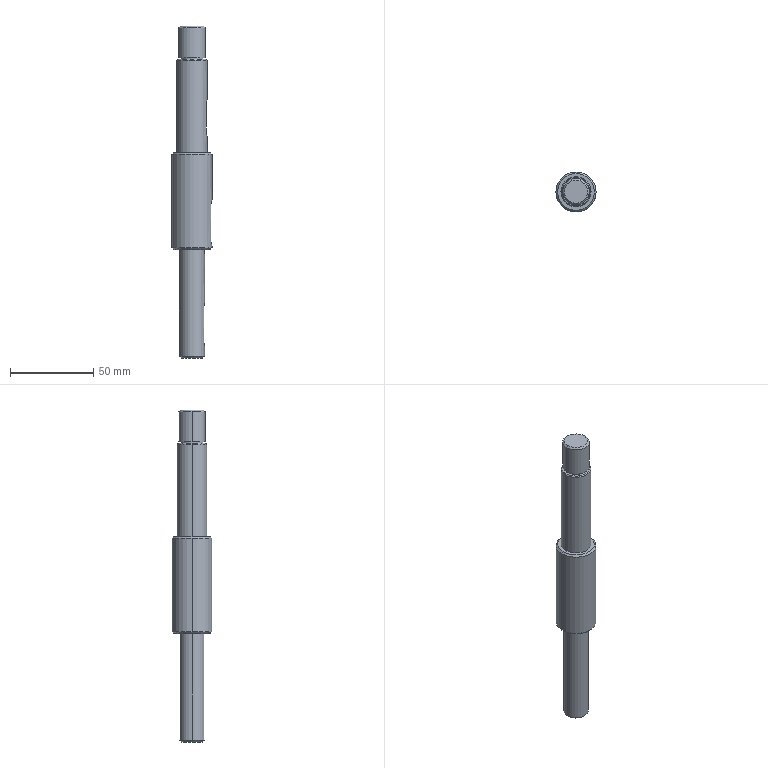Part | SolidWorks | features ICE 8, Chamfer 5, MoveFace 2, Cut 1, Revolution 1 | 1 solid | 44 faces | box 24 x 24 x 199 mm | volume 54258 mm3 | cylinder 19 | plane 15 | cone 10 | commonest cylinder face diameters 5 x3 6 x3 8 x3 13.5 x2 15 x2 16 x2
STEP:
#1=CARTESIAN_POINT('',(4.5,0.,-191.5));
#2=VERTEX_POINT('',#1);
#3=CARTESIAN_POINT('',(4.5,2.5,-189.));
#4=VERTEX_POINT('',#3);
#5=CARTESIAN_POINT('',(4.5,0.,-189.));
#6=DIRECTION('',(1.,0.,0.));
#7=DIRECTION('',(0.,0.,-1.));
#8=AXIS2_PLACEMENT_3D('',#5,#6,#7);
#9=CIRCLE('',#8,2.5);
#10=EDGE_CURVE('',#2,#4,#9,.T.);
#11=ORIENTED_EDGE('',*,*,#10,.F.);
#12=CARTESIAN_POINT('',(7.5,0.,-191.5));
#13=VERTEX_POINT('',#12);
#14=CARTESIAN_POINT('',(4.5,0.,-191.5));
#15=DIRECTION('',(1.,0.,0.));
#16=VECTOR('',#15,1000.);
#17=LINE('',#14,#16);
#18=EDGE_CURVE('',#2,#13,#17,.T.);
#19=ORIENTED_EDGE('',*,*,#18,.T.);
#20=CARTESIAN_POINT('',(7.071,2.5,-189.));
#21=VERTEX_POINT('',#20);
#22=CARTESIAN_POINT('',(7.5,0.,-191.5));
#23=CARTESIAN_POINT('',(7.5,0.1643,-191.5));
#24=CARTESIAN_POINT('',(7.494,0.3311,-191.483));
#25=CARTESIAN_POINT('',(7.473,0.6524,-191.419));
#26=CARTESIAN_POINT('',(7.458,0.8088,-191.371));
#27=CARTESIAN_POINT('',(7.419,1.113,-191.245));
#28=CARTESIAN_POINT('',(7.395,1.257,-191.167));
#29=CARTESIAN_POINT('',(7.344,1.526,-190.987));
#30=CARTESIAN_POINT('',(7.316,1.653,-190.882));
#31=CARTESIAN_POINT('',(7.261,1.883,-190.652));
#32=CARTESIAN_POINT('',(7.233,1.986,-190.527));
#33=CARTESIAN_POINT('',(7.181,2.167,-190.258));
#34=CARTESIAN_POINT('',(7.156,2.245,-190.112));
#35=CARTESIAN_POINT('',(7.116,2.37,-189.811));
#36=CARTESIAN_POINT('',(7.1,2.418,-189.656));
#37=CARTESIAN_POINT('',(7.077,2.483,-189.332));
#38=CARTESIAN_POINT('',(7.071,2.5,-189.166));
#39=CARTESIAN_POINT('',(7.071,2.5,-189.));
#40=B_SPLINE_CURVE_WITH_KNOTS('',3,(#22,#23,#24,#25,#26,#27,#28,#29,#30,#31,#32,#33,#34,#35,#36,#37,#38,#39),.UNSPECIFIED.,.F.,.F.,(4,2,2,2,2,2,2,2,4),(0.003937,0.004429,0.004921,0.005412,0.005904,0.006395,0.006887,0.007378,0.00787),.UNSPECIFIED.);
#41=EDGE_CURVE('',#13,#21,#40,.T.);
#42=ORIENTED_EDGE('',*,*,#41,.T.);
#43=CARTESIAN_POINT('',(4.5,2.5,-189.));
#44=DIRECTION('',(1.,0.,0.));
#45=VECTOR('',#44,1000.);
#46=LINE('',#43,#45);
#47=EDGE_CURVE('',#4,#21,#46,.T.);
#48=ORIENTED_EDGE('',*,*,#47,.F.);
#49=EDGE_LOOP('',(#11,#19,#42,#48));
#50=FACE_OUTER_BOUND('',#49,.T.);
#51=CARTESIAN_POINT('',(4.5,0.,-189.));
#52=DIRECTION('',(1.,0.,0.));
#53=DIRECTION('',(0.,0.,-1.));
#54=AXIS2_PLACEMENT_3D('',#51,#52,#53);
#55=CYLINDRICAL_SURFACE('',#54,2.5);
#56=ADVANCED_FACE('',(#50),#55,.F.);
#57=CARTESIAN_POINT('',(-6.5,0.,-199.));
#58=VERTEX_POINT('',#57);
#59=CARTESIAN_POINT('',(6.5,0.,-199.));
#60=VERTEX_POINT('',#59);
#61=CARTESIAN_POINT('',(0.,0.,-199.));
#62=DIRECTION('',(0.,0.,-1.));
#63=DIRECTION('',(1.,0.,0.));
#64=AXIS2_PLACEMENT_3D('',#61,#62,#63);
#65=CIRCLE('',#64,6.5);
#66=EDGE_CURVE('',#58,#60,#65,.T.);
#67=ORIENTED_EDGE('',*,*,#66,.F.);
#68=CARTESIAN_POINT('',(-7.5,0.,-198.));
#69=VERTEX_POINT('',#68);
#70=CARTESIAN_POINT('',(-7.5,0.,-198.));
#71=DIRECTION('',(-0.7071,0.,0.7071));
#72=VECTOR('',#71,1000.);
#73=LINE('',#70,#72);
#74=EDGE_CURVE('',#58,#69,#73,.T.);
#75=ORIENTED_EDGE('',*,*,#74,.T.);
#76=CARTESIAN_POINT('',(7.5,0.,-198.));
#77=VERTEX_POINT('',#76);
#78=CARTESIAN_POINT('',(0.,0.,-198.));
#79=DIRECTION('',(0.,0.,1.));
#80=DIRECTION('',(1.,0.,0.));
#81=AXIS2_PLACEMENT_3D('',#78,#79,#80);
#82=CIRCLE('',#81,7.5);
#83=EDGE_CURVE('',#77,#69,#82,.T.);
#84=ORIENTED_EDGE('',*,*,#83,.F.);
#85=CARTESIAN_POINT('',(7.5,0.,-198.));
#86=DIRECTION('',(0.7071,0.,0.7071));
#87=VECTOR('',#86,1000.);
#88=LINE('',#85,#87);
#89=EDGE_CURVE('',#60,#77,#88,.T.);
#90=ORIENTED_EDGE('',*,*,#89,.F.);
#91=EDGE_LOOP('',(#67,#75,#84,#90));
#92=FACE_OUTER_BOUND('',#91,.T.);
#93=CARTESIAN_POINT('',(0.,0.,-198.));
#94=DIRECTION('',(0.,0.,1.));
#95=DIRECTION('',(1.,0.,0.));
#96=AXIS2_PLACEMENT_3D('',#93,#94,#95);
#97=CONICAL_SURFACE('',#96,7.5,0.7854);
#98=ADVANCED_FACE('',(#92),#97,.T.);
#99=CARTESIAN_POINT('',(7.5,0.,-134.));
#100=VERTEX_POINT('',#99);
#101=CARTESIAN_POINT('',(-7.5,0.,-134.));
#102=VERTEX_POINT('',#101);
#103=CARTESIAN_POINT('',(0.,0.,-134.));
#104=DIRECTION('',(0.,0.,1.));
#105=DIRECTION('',(-1.,0.,0.));
#106=AXIS2_PLACEMENT_3D('',#103,#104,#105);
#107=CIRCLE('',#106,7.5);
#108=EDGE_CURVE('',#100,#102,#107,.T.);
#109=ORIENTED_EDGE('',*,*,#108,.F.);
#110=CARTESIAN_POINT('',(7.5,0.,-166.5));
#111=VERTEX_POINT('',#110);
#112=CARTESIAN_POINT('',(7.5,0.,-105.716));
#113=DIRECTION('',(0.,0.,-1.));
#114=VECTOR('',#113,1000.);
#115=LINE('',#112,#114);
#116=EDGE_CURVE('',#100,#111,#115,.T.);
#117=ORIENTED_EDGE('',*,*,#116,.T.);
#118=CARTESIAN_POINT('',(7.071,2.5,-169.));
#119=VERTEX_POINT('',#118);
#120=CARTESIAN_POINT('',(7.071,2.5,-169.));
#121=CARTESIAN_POINT('',(7.071,2.5,-168.833));
#122=CARTESIAN_POINT('',(7.077,2.484,-168.67));
#123=CARTESIAN_POINT('',(7.099,2.419,-168.349));
#124=CARTESIAN_POINT('',(7.116,2.371,-168.189));
#125=CARTESIAN_POINT('',(7.157,2.245,-167.887));
#126=CARTESIAN_POINT('',(7.181,2.168,-167.744));
#127=CARTESIAN_POINT('',(7.233,1.986,-167.473));
#128=CARTESIAN_POINT('',(7.261,1.882,-167.346));
#129=CARTESIAN_POINT('',(7.344,1.538,-167.003));
#130=CARTESIAN_POINT('',(7.399,1.261,-166.817));
#131=CARTESIAN_POINT('',(7.458,0.81,-166.629));
#132=CARTESIAN_POINT('',(7.473,0.6511,-166.581));
#133=CARTESIAN_POINT('',(7.495,0.3276,-166.516));
#134=CARTESIAN_POINT('',(7.5,0.1645,-166.5));
#135=CARTESIAN_POINT('',(7.5,0.,-166.5));
#136=B_SPLINE_CURVE_WITH_KNOTS('',3,(#120,#121,#122,#123,#124,#125,#126,#127,#128,#129,#130,#131,#132,#133,#134,#135),.UNSPECIFIED.,.F.,.F.,(4,2,2,2,2,2,2,4),(0.,0.0004922,0.0009844,0.001477,0.001969,0.002953,0.003445,0.003937),.UNSPECIFIED.);
#137=EDGE_CURVE('',#119,#111,#136,.T.);
#138=ORIENTED_EDGE('',*,*,#137,.F.);
#139=CARTESIAN_POINT('',(7.071,2.5,-105.716));
#140=DIRECTION('',(0.,0.,1.));
#141=VECTOR('',#140,1000.);
#142=LINE('',#139,#141);
#143=EDGE_CURVE('',#21,#119,#142,.T.);
#144=ORIENTED_EDGE('',*,*,#143,.F.);
#145=ORIENTED_EDGE('',*,*,#41,.F.);
#146=CARTESIAN_POINT('',(7.5,0.,-105.716));
#147=DIRECTION('',(0.,0.,-1.));
#148=VECTOR('',#147,1000.);
#149=LINE('',#146,#148);
#150=EDGE_CURVE('',#13,#77,#149,.T.);
#151=ORIENTED_EDGE('',*,*,#150,.T.);
#152=ORIENTED_EDGE('',*,*,#83,.T.);
#153=CARTESIAN_POINT('',(-7.5,0.,-105.716));
#154=DIRECTION('',(0.,0.,-1.));
#155=VECTOR('',#154,1000.);
#156=LINE('',#153,#155);
#157=EDGE_CURVE('',#102,#69,#156,.T.);
#158=ORIENTED_EDGE('',*,*,#157,.F.);
#159=EDGE_LOOP('',(#109,#117,#138,#144,#145,#151,#152,#158));
#160=FACE_OUTER_BOUND('',#159,.T.);
#161=CARTESIAN_POINT('',(0.,0.,-105.716));
#162=DIRECTION('',(0.,0.,-1.));
#163=DIRECTION('',(-1.,0.,0.));
#164=AXIS2_PLACEMENT_3D('',#161,#162,#163);
#165=CYLINDRICAL_SURFACE('',#164,7.5);
#166=ADVANCED_FACE('',(#160),#165,.T.);
#167=CARTESIAN_POINT('',(11.,0.,-76.));
#168=VERTEX_POINT('',#167);
#169=CARTESIAN_POINT('',(-11.,0.,-76.));
#170=VERTEX_POINT('',#169);
#171=CARTESIAN_POINT('',(0.,0.,-76.));
#172=DIRECTION('',(0.,0.,1.));
#173=DIRECTION('',(1.,0.,0.));
#174=AXIS2_PLACEMENT_3D('',#171,#172,#173);
#175=CIRCLE('',#174,11.);
#176=EDGE_CURVE('',#168,#170,#175,.T.);
#177=ORIENTED_EDGE('',*,*,#176,.F.);
#178=CARTESIAN_POINT('',(12.,0.,-77.));
#179=VERTEX_POINT('',#178);
#180=CARTESIAN_POINT('',(11.,0.,-76.));
#181=DIRECTION('',(0.7071,0.,-0.7071));
#182=VECTOR('',#181,1000.);
#183=LINE('',#180,#182);
#184=EDGE_CURVE('',#168,#179,#183,.T.);
#185=ORIENTED_EDGE('',*,*,#184,.T.);
#186=CARTESIAN_POINT('',(-12.,0.,-77.));
#187=VERTEX_POINT('',#186);
#188=CARTESIAN_POINT('',(0.,0.,-77.));
#189=DIRECTION('',(0.,0.,-1.));
#190=DIRECTION('',(1.,0.,0.));
#191=AXIS2_PLACEMENT_3D('',#188,#189,#190);
#192=CIRCLE('',#191,12.);
#193=EDGE_CURVE('',#187,#179,#192,.T.);
#194=ORIENTED_EDGE('',*,*,#193,.F.);
#195=CARTESIAN_POINT('',(-11.,0.,-76.));
#196=DIRECTION('',(-0.7071,0.,-0.7071));
#197=VECTOR('',#196,1000.);
#198=LINE('',#195,#197);
#199=EDGE_CURVE('',#170,#187,#198,.T.);
#200=ORIENTED_EDGE('',*,*,#199,.F.);
#201=EDGE_LOOP('',(#177,#185,#194,#200));
#202=FACE_OUTER_BOUND('',#201,.T.);
#203=CARTESIAN_POINT('',(0.,0.,-76.));
#204=DIRECTION('',(0.,0.,-1.));
#205=DIRECTION('',(-1.,0.,0.));
#206=AXIS2_PLACEMENT_3D('',#203,#204,#205);
#207=CONICAL_SURFACE('',#206,11.,0.7854);
#208=ADVANCED_FACE('',(#202),#207,.T.);
#209=CARTESIAN_POINT('',(12.,0.,-133.));
#210=VERTEX_POINT('',#209);
#211=CARTESIAN_POINT('',(-12.,0.,-133.));
#212=VERTEX_POINT('',#211);
#213=CARTESIAN_POINT('',(0.,0.,-133.));
#214=DIRECTION('',(0.,0.,1.));
#215=DIRECTION('',(-1.,0.,0.));
#216=AXIS2_PLACEMENT_3D('',#213,#214,#215);
#217=CIRCLE('',#216,12.);
#218=EDGE_CURVE('',#210,#212,#217,.T.);
#219=ORIENTED_EDGE('',*,*,#218,.T.);
#220=CARTESIAN_POINT('',(-12.,0.,0.));
#221=DIRECTION('',(0.,0.,1.));
#222=VECTOR('',#221,1000.);
#223=LINE('',#220,#222);
#224=EDGE_CURVE('',#212,#187,#223,.T.);
#225=ORIENTED_EDGE('',*,*,#224,.T.);
#226=ORIENTED_EDGE('',*,*,#193,.T.);
#227=CARTESIAN_POINT('',(12.,0.,-104.));
#228=VERTEX_POINT('',#227);
#229=CARTESIAN_POINT('',(12.,0.,0.));
#230=DIRECTION('',(0.,0.,1.));
#231=VECTOR('',#230,1000.);
#232=LINE('',#229,#231);
#233=EDGE_CURVE('',#228,#179,#232,.T.);
#234=ORIENTED_EDGE('',*,*,#233,.F.);
#235=CARTESIAN_POINT('',(11.314,4.,-108.));
#236=VERTEX_POINT('',#235);
#237=CARTESIAN_POINT('',(12.,0.,-104.));
#238=CARTESIAN_POINT('',(12.,0.2628,-104.));
#239=CARTESIAN_POINT('',(11.991,0.5297,-104.027));
#240=CARTESIAN_POINT('',(11.957,1.044,-104.13));
#241=CARTESIAN_POINT('',(11.933,1.294,-104.206));
#242=CARTESIAN_POINT('',(11.87,1.78,-104.408));
#243=CARTESIAN_POINT('',(11.832,2.011,-104.533));
#244=CARTESIAN_POINT('',(11.751,2.442,-104.821));
#245=CARTESIAN_POINT('',(11.706,2.645,-104.988));
#246=CARTESIAN_POINT('',(11.617,3.013,-105.356));
#247=CARTESIAN_POINT('',(11.573,3.177,-105.556));
#248=CARTESIAN_POINT('',(11.489,3.467,-105.987));
#249=CARTESIAN_POINT('',(11.45,3.592,-106.221));
#250=CARTESIAN_POINT('',(11.385,3.792,-106.702));
#251=CARTESIAN_POINT('',(11.359,3.869,-106.951));
#252=CARTESIAN_POINT('',(11.323,3.973,-107.468));
#253=CARTESIAN_POINT('',(11.314,4.,-107.734));
#254=CARTESIAN_POINT('',(11.314,4.,-108.));
#255=B_SPLINE_CURVE_WITH_KNOTS('',3,(#237,#238,#239,#240,#241,#242,#243,#244,#245,#246,#247,#248,#249,#250,#251,#252,#253,#254),.UNSPECIFIED.,.F.,.F.,(4,2,2,2,2,2,2,2,4),(0.0063,0.007086,0.007873,0.008659,0.009446,0.01023,0.01102,0.01181,0.01259),.UNSPECIFIED.);
#256=EDGE_CURVE('',#228,#236,#255,.T.);
#257=ORIENTED_EDGE('',*,*,#256,.T.);
#258=CARTESIAN_POINT('',(11.314,4.,-128.));
#259=VERTEX_POINT('',#258);
#260=CARTESIAN_POINT('',(11.314,4.,0.));
#261=DIRECTION('',(0.,0.,-1.));
#262=VECTOR('',#261,1000.);
#263=LINE('',#260,#262);
#264=EDGE_CURVE('',#236,#259,#263,.T.);
#265=ORIENTED_EDGE('',*,*,#264,.T.);
#266=CARTESIAN_POINT('',(12.,0.,-132.));
#267=VERTEX_POINT('',#266);
#268=CARTESIAN_POINT('',(11.314,4.,-128.));
#269=CARTESIAN_POINT('',(11.314,4.,-128.266));
#270=CARTESIAN_POINT('',(11.323,3.974,-128.528));
#271=CARTESIAN_POINT('',(11.359,3.871,-129.042));
#272=CARTESIAN_POINT('',(11.385,3.793,-129.297));
#273=CARTESIAN_POINT('',(11.45,3.591,-129.781));
#274=CARTESIAN_POINT('',(11.489,3.468,-130.01));
#275=CARTESIAN_POINT('',(11.573,3.178,-130.443));
#276=CARTESIAN_POINT('',(11.618,3.01,-130.647));
#277=CARTESIAN_POINT('',(11.707,2.644,-131.013));
#278=CARTESIAN_POINT('',(11.751,2.444,-131.178));
#279=CARTESIAN_POINT('',(11.833,2.007,-131.47));
#280=CARTESIAN_POINT('',(11.87,1.777,-131.593));
#281=CARTESIAN_POINT('',(11.932,1.296,-131.793));
#282=CARTESIAN_POINT('',(11.958,1.042,-131.871));
#283=CARTESIAN_POINT('',(11.991,0.5242,-131.974));
#284=CARTESIAN_POINT('',(12.,0.2632,-132.));
#285=CARTESIAN_POINT('',(12.,0.,-132.));
#286=B_SPLINE_CURVE_WITH_KNOTS('',3,(#268,#269,#270,#271,#272,#273,#274,#275,#276,#277,#278,#279,#280,#281,#282,#283,#284,#285),.UNSPECIFIED.,.F.,.F.,(4,2,2,2,2,2,2,2,4),(0.,0.0007875,0.001575,0.002362,0.00315,0.003937,0.004725,0.005512,0.0063),.UNSPECIFIED.);
#287=EDGE_CURVE('',#259,#267,#286,.T.);
#288=ORIENTED_EDGE('',*,*,#287,.T.);
#289=CARTESIAN_POINT('',(12.,0.,0.));
#290=DIRECTION('',(0.,0.,1.));
#291=VECTOR('',#290,1000.);
#292=LINE('',#289,#291);
#293=EDGE_CURVE('',#210,#267,#292,.T.);
#294=ORIENTED_EDGE('',*,*,#293,.F.);
#295=EDGE_LOOP('',(#219,#225,#226,#234,#257,#265,#288,#294));
#296=FACE_OUTER_BOUND('',#295,.T.);
#297=CARTESIAN_POINT('',(0.,0.,0.));
#298=DIRECTION('',(0.,0.,1.));
#299=DIRECTION('',(1.,0.,0.));
#300=AXIS2_PLACEMENT_3D('',#297,#298,#299);
#301=CYLINDRICAL_SURFACE('',#300,12.);
#302=ADVANCED_FACE('',(#296),#301,.T.);
#303=CARTESIAN_POINT('',(8.,0.,-132.));
#304=VERTEX_POINT('',#303);
#305=CARTESIAN_POINT('',(8.,4.,-128.));
#306=VERTEX_POINT('',#305);
#307=CARTESIAN_POINT('',(8.,0.,-128.));
#308=DIRECTION('',(1.,0.,0.));
#309=DIRECTION('',(0.,0.,-1.));
#310=AXIS2_PLACEMENT_3D('',#307,#308,#309);
#311=CIRCLE('',#310,4.);
#312=EDGE_CURVE('',#304,#306,#311,.T.);
#313=ORIENTED_EDGE('',*,*,#312,.F.);
#314=CARTESIAN_POINT('',(8.,0.,-132.));
#315=DIRECTION('',(1.,0.,0.));
#316=VECTOR('',#315,1000.);
#317=LINE('',#314,#316);
#318=EDGE_CURVE('',#304,#267,#317,.T.);
#319=ORIENTED_EDGE('',*,*,#318,.T.);
#320=ORIENTED_EDGE('',*,*,#287,.F.);
#321=CARTESIAN_POINT('',(8.,4.,-128.));
#322=DIRECTION('',(1.,0.,0.));
#323=VECTOR('',#322,1000.);
#324=LINE('',#321,#323);
#325=EDGE_CURVE('',#306,#259,#324,.T.);
#326=ORIENTED_EDGE('',*,*,#325,.F.);
#327=EDGE_LOOP('',(#313,#319,#320,#326));
#328=FACE_OUTER_BOUND('',#327,.T.);
#329=CARTESIAN_POINT('',(8.,0.,-128.));
#330=DIRECTION('',(1.,0.,0.));
#331=DIRECTION('',(0.,0.,-1.));
#332=AXIS2_PLACEMENT_3D('',#329,#330,#331);
#333=CYLINDRICAL_SURFACE('',#332,4.);
#334=ADVANCED_FACE('',(#328),#333,.F.);
#335=CARTESIAN_POINT('',(-11.,0.,-134.));
#336=VERTEX_POINT('',#335);
#337=CARTESIAN_POINT('',(11.,0.,-134.));
#338=VERTEX_POINT('',#337);
#339=CARTESIAN_POINT('',(0.,0.,-134.));
#340=DIRECTION('',(0.,0.,-1.));
#341=DIRECTION('',(-1.,0.,0.));
#342=AXIS2_PLACEMENT_3D('',#339,#340,#341);
#343=CIRCLE('',#342,11.);
#344=EDGE_CURVE('',#336,#338,#343,.T.);
#345=ORIENTED_EDGE('',*,*,#344,.F.);
#346=CARTESIAN_POINT('',(-11.,0.,-134.));
#347=DIRECTION('',(-0.7071,0.,0.7071));
#348=VECTOR('',#347,1000.);
#349=LINE('',#346,#348);
#350=EDGE_CURVE('',#336,#212,#349,.T.);
#351=ORIENTED_EDGE('',*,*,#350,.T.);
#352=ORIENTED_EDGE('',*,*,#218,.F.);
#353=CARTESIAN_POINT('',(11.,0.,-134.));
#354=DIRECTION('',(0.7071,0.,0.7071));
#355=VECTOR('',#354,1000.);
#356=LINE('',#353,#355);
#357=EDGE_CURVE('',#338,#210,#356,.T.);
#358=ORIENTED_EDGE('',*,*,#357,.F.);
#359=EDGE_LOOP('',(#345,#351,#352,#358));
#360=FACE_OUTER_BOUND('',#359,.T.);
#361=CARTESIAN_POINT('',(0.,0.,-134.));
#362=DIRECTION('',(0.,0.,1.));
#363=DIRECTION('',(1.,0.,0.));
#364=AXIS2_PLACEMENT_3D('',#361,#362,#363);
#365=CONICAL_SURFACE('',#364,11.,0.7854);
#366=ADVANCED_FACE('',(#360),#365,.T.);
#367=CARTESIAN_POINT('',(9.,0.,-76.));
#368=VERTEX_POINT('',#367);
#369=CARTESIAN_POINT('',(-9.,0.,-76.));
#370=VERTEX_POINT('',#369);
#371=CARTESIAN_POINT('',(0.,0.,-76.));
#372=DIRECTION('',(0.,0.,1.));
#373=DIRECTION('',(1.,0.,0.));
#374=AXIS2_PLACEMENT_3D('',#371,#372,#373);
#375=CIRCLE('',#374,9.);
#376=EDGE_CURVE('',#368,#370,#375,.T.);
#377=ORIENTED_EDGE('',*,*,#376,.T.);
#378=CARTESIAN_POINT('',(-9.,0.,-20.5));
#379=VERTEX_POINT('',#378);
#380=CARTESIAN_POINT('',(-9.,0.,0.));
#381=DIRECTION('',(0.,0.,1.));
#382=VECTOR('',#381,1000.);
#383=LINE('',#380,#382);
#384=EDGE_CURVE('',#370,#379,#383,.T.);
#385=ORIENTED_EDGE('',*,*,#384,.T.);
#386=CARTESIAN_POINT('',(9.,0.,-20.5));
#387=VERTEX_POINT('',#386);
#388=CARTESIAN_POINT('',(0.,0.,-20.5));
#389=DIRECTION('',(0.,0.,-1.));
#390=DIRECTION('',(-1.,0.,0.));
#391=AXIS2_PLACEMENT_3D('',#388,#389,#390);
#392=CIRCLE('',#391,9.);
#393=EDGE_CURVE('',#379,#387,#392,.T.);
#394=ORIENTED_EDGE('',*,*,#393,.T.);
#395=CARTESIAN_POINT('',(9.,0.,-44.));
#396=VERTEX_POINT('',#395);
#397=CARTESIAN_POINT('',(9.,0.,0.));
#398=DIRECTION('',(0.,0.,1.));
#399=VECTOR('',#398,1000.);
#400=LINE('',#397,#399);
#401=EDGE_CURVE('',#396,#387,#400,.T.);
#402=ORIENTED_EDGE('',*,*,#401,.F.);
#403=CARTESIAN_POINT('',(8.485,3.,-47.));
#404=VERTEX_POINT('',#403);
#405=CARTESIAN_POINT('',(9.,0.,-44.));
#406=CARTESIAN_POINT('',(9.,0.1971,-44.));
#407=CARTESIAN_POINT('',(8.993,0.3973,-44.02));
#408=CARTESIAN_POINT('',(8.968,0.7829,-44.097));
#409=CARTESIAN_POINT('',(8.949,0.9705,-44.154));
#410=CARTESIAN_POINT('',(8.902,1.335,-44.306));
#411=CARTESIAN_POINT('',(8.874,1.508,-44.399));
#412=CARTESIAN_POINT('',(8.813,1.831,-44.616));
#413=CARTESIAN_POINT('',(8.78,1.984,-44.741));
#414=CARTESIAN_POINT('',(8.713,2.26,-45.017));
#415=CARTESIAN_POINT('',(8.68,2.383,-45.167));
#416=CARTESIAN_POINT('',(8.617,2.6,-45.491));
#417=CARTESIAN_POINT('',(8.588,2.694,-45.666));
#418=CARTESIAN_POINT('',(8.539,2.844,-46.026));
#419=CARTESIAN_POINT('',(8.519,2.902,-46.213));
#420=CARTESIAN_POINT('',(8.492,2.98,-46.601));
#421=CARTESIAN_POINT('',(8.485,3.,-46.8));
#422=CARTESIAN_POINT('',(8.485,3.,-47.));
#423=B_SPLINE_CURVE_WITH_KNOTS('',3,(#405,#406,#407,#408,#409,#410,#411,#412,#413,#414,#415,#416,#417,#418,#419,#420,#421,#422),.UNSPECIFIED.,.F.,.F.,(4,2,2,2,2,2,2,2,4),(0.004725,0.005315,0.005905,0.006494,0.007084,0.007674,0.008264,0.008854,0.009444),.UNSPECIFIED.);
#424=EDGE_CURVE('',#396,#404,#423,.T.);
#425=ORIENTED_EDGE('',*,*,#424,.T.);
#426=CARTESIAN_POINT('',(8.485,3.,-63.));
#427=VERTEX_POINT('',#426);
#428=CARTESIAN_POINT('',(8.485,3.,0.));
#429=DIRECTION('',(0.,0.,-1.));
#430=VECTOR('',#429,1000.);
#431=LINE('',#428,#430);
#432=EDGE_CURVE('',#404,#427,#431,.T.);
#433=ORIENTED_EDGE('',*,*,#432,.T.);
#434=CARTESIAN_POINT('',(9.,0.,-66.));
#435=VERTEX_POINT('',#434);
#436=CARTESIAN_POINT('',(8.485,3.,-63.));
#437=CARTESIAN_POINT('',(8.485,3.,-63.2));
#438=CARTESIAN_POINT('',(8.492,2.98,-63.396));
#439=CARTESIAN_POINT('',(8.519,2.903,-63.781));
#440=CARTESIAN_POINT('',(8.539,2.845,-63.973));
#441=CARTESIAN_POINT('',(8.588,2.694,-64.335));
#442=CARTESIAN_POINT('',(8.617,2.601,-64.507));
#443=CARTESIAN_POINT('',(8.679,2.384,-64.832));
#444=CARTESIAN_POINT('',(8.713,2.258,-64.985));
#445=CARTESIAN_POINT('',(8.813,1.846,-65.397));
#446=CARTESIAN_POINT('',(8.879,1.513,-65.62));
#447=CARTESIAN_POINT('',(8.949,0.972,-65.845));
#448=CARTESIAN_POINT('',(8.968,0.7813,-65.903));
#449=CARTESIAN_POINT('',(8.994,0.3931,-65.981));
#450=CARTESIAN_POINT('',(9.,0.1974,-66.));
#451=CARTESIAN_POINT('',(9.,0.,-66.));
#452=B_SPLINE_CURVE_WITH_KNOTS('',3,(#436,#437,#438,#439,#440,#441,#442,#443,#444,#445,#446,#447,#448,#449,#450,#451),.UNSPECIFIED.,.F.,.F.,(4,2,2,2,2,2,2,4),(0.,0.0005906,0.001181,0.001772,0.002362,0.003544,0.004134,0.004725),.UNSPECIFIED.);
#453=EDGE_CURVE('',#427,#435,#452,.T.);
#454=ORIENTED_EDGE('',*,*,#453,.T.);
#455=CARTESIAN_POINT('',(9.,0.,0.));
#456=DIRECTION('',(0.,0.,1.));
#457=VECTOR('',#456,1000.);
#458=LINE('',#455,#457);
#459=EDGE_CURVE('',#368,#435,#458,.T.);
#460=ORIENTED_EDGE('',*,*,#459,.F.);
#461=EDGE_LOOP('',(#377,#385,#394,#402,#425,#433,#454,#460));
#462=FACE_OUTER_BOUND('',#461,.T.);
#463=CARTESIAN_POINT('',(0.,0.,0.));
#464=DIRECTION('',(0.,0.,1.));
#465=DIRECTION('',(1.,0.,0.));
#466=AXIS2_PLACEMENT_3D('',#463,#464,#465);
#467=CYLINDRICAL_SURFACE('',#466,9.);
#468=ADVANCED_FACE('',(#462),#467,.T.);
#469=CARTESIAN_POINT('',(8.5,0.,-20.));
#470=VERTEX_POINT('',#469);
#471=CARTESIAN_POINT('',(-8.5,0.,-20.));
#472=VERTEX_POINT('',#471);
#473=CARTESIAN_POINT('',(0.,0.,-20.));
#474=DIRECTION('',(0.,0.,1.));
#475=DIRECTION('',(-1.,0.,0.));
#476=AXIS2_PLACEMENT_3D('',#473,#474,#475);
#477=CIRCLE('',#476,8.5);
#478=EDGE_CURVE('',#470,#472,#477,.T.);
#479=ORIENTED_EDGE('',*,*,#478,.F.);
#480=CARTESIAN_POINT('',(8.5,0.,-20.));
#481=DIRECTION('',(0.7071,0.,-0.7071));
#482=VECTOR('',#481,1000.);
#483=LINE('',#480,#482);
#484=EDGE_CURVE('',#470,#387,#483,.T.);
#485=ORIENTED_EDGE('',*,*,#484,.T.);
#486=ORIENTED_EDGE('',*,*,#393,.F.);
#487=CARTESIAN_POINT('',(-8.5,0.,-20.));
#488=DIRECTION('',(-0.7071,0.,-0.7071));
#489=VECTOR('',#488,1000.);
#490=LINE('',#487,#489);
#491=EDGE_CURVE('',#472,#379,#490,.T.);
#492=ORIENTED_EDGE('',*,*,#491,.F.);
#493=EDGE_LOOP('',(#479,#485,#486,#492));
#494=FACE_OUTER_BOUND('',#493,.T.);
#495=CARTESIAN_POINT('',(0.,0.,-20.));
#496=DIRECTION('',(0.,0.,-1.));
#497=DIRECTION('',(-1.,0.,0.));
#498=AXIS2_PLACEMENT_3D('',#495,#496,#497);
#499=CONICAL_SURFACE('',#498,8.5,0.7854);
#500=ADVANCED_FACE('',(#494),#499,.T.);
#501=CARTESIAN_POINT('',(6.75,0.,-20.));
#502=VERTEX_POINT('',#501);
#503=CARTESIAN_POINT('',(-6.75,0.,-20.));
#504=VERTEX_POINT('',#503);
#505=CARTESIAN_POINT('',(0.,0.,-20.));
#506=DIRECTION('',(0.,0.,1.));
#507=DIRECTION('',(1.,0.,0.));
#508=AXIS2_PLACEMENT_3D('',#505,#506,#507);
#509=CIRCLE('',#508,6.75);
#510=EDGE_CURVE('',#502,#504,#509,.T.);
#511=ORIENTED_EDGE('',*,*,#510,.T.);
#512=CARTESIAN_POINT('',(-6.75,0.,-19.));
#513=VERTEX_POINT('',#512);
#514=CARTESIAN_POINT('',(-6.75,0.,0.));
#515=DIRECTION('',(0.,0.,1.));
#516=VECTOR('',#515,1000.);
#517=LINE('',#514,#516);
#518=EDGE_CURVE('',#504,#513,#517,.T.);
#519=ORIENTED_EDGE('',*,*,#518,.T.);
#520=CARTESIAN_POINT('',(6.75,0.,-19.));
#521=VERTEX_POINT('',#520);
#522=CARTESIAN_POINT('',(0.,0.,-19.));
#523=DIRECTION('',(0.,0.,1.));
#524=DIRECTION('',(1.,0.,0.));
#525=AXIS2_PLACEMENT_3D('',#522,#523,#524);
#526=CIRCLE('',#525,6.75);
#527=EDGE_CURVE('',#521,#513,#526,.T.);
#528=ORIENTED_EDGE('',*,*,#527,.F.);
#529=CARTESIAN_POINT('',(6.75,0.,0.));
#530=DIRECTION('',(0.,0.,1.));
#531=VECTOR('',#530,1000.);
#532=LINE('',#529,#531);
#533=EDGE_CURVE('',#502,#521,#532,.T.);
#534=ORIENTED_EDGE('',*,*,#533,.F.);
#535=EDGE_LOOP('',(#511,#519,#528,#534));
#536=FACE_OUTER_BOUND('',#535,.T.);
#537=CARTESIAN_POINT('',(0.,0.,0.));
#538=DIRECTION('',(0.,0.,1.));
#539=DIRECTION('',(1.,0.,0.));
#540=AXIS2_PLACEMENT_3D('',#537,#538,#539);
#541=CYLINDRICAL_SURFACE('',#540,6.75);
#542=ADVANCED_FACE('',(#536),#541,.T.);
#543=CARTESIAN_POINT('',(8.,0.,-19.));
#544=VERTEX_POINT('',#543);
#545=CARTESIAN_POINT('',(-8.,0.,-19.));
#546=VERTEX_POINT('',#545);
#547=CARTESIAN_POINT('',(0.,0.,-19.));
#548=DIRECTION('',(0.,0.,1.));
#549=DIRECTION('',(1.,0.,0.));
#550=AXIS2_PLACEMENT_3D('',#547,#548,#549);
#551=CIRCLE('',#550,8.);
#552=EDGE_CURVE('',#544,#546,#551,.T.);
#553=ORIENTED_EDGE('',*,*,#552,.T.);
#554=CARTESIAN_POINT('',(-8.,0.,-1.));
#555=VERTEX_POINT('',#554);
#556=CARTESIAN_POINT('',(-8.,0.,0.));
#557=DIRECTION('',(0.,0.,1.));
#558=VECTOR('',#557,1000.);
#559=LINE('',#556,#558);
#560=EDGE_CURVE('',#546,#555,#559,.T.);
#561=ORIENTED_EDGE('',*,*,#560,.T.);
#562=CARTESIAN_POINT('',(8.,0.,-1.));
#563=VERTEX_POINT('',#562);
#564=CARTESIAN_POINT('',(0.,0.,-1.));
#565=DIRECTION('',(0.,0.,-1.));
#566=DIRECTION('',(-1.,0.,0.));
#567=AXIS2_PLACEMENT_3D('',#564,#565,#566);
#568=CIRCLE('',#567,8.);
#569=EDGE_CURVE('',#555,#563,#568,.T.);
#570=ORIENTED_EDGE('',*,*,#569,.T.);
#571=CARTESIAN_POINT('',(8.,0.,0.));
#572=DIRECTION('',(0.,0.,1.));
#573=VECTOR('',#572,1000.);
#574=LINE('',#571,#573);
#575=EDGE_CURVE('',#544,#563,#574,.T.);
#576=ORIENTED_EDGE('',*,*,#575,.F.);
#577=EDGE_LOOP('',(#553,#561,#570,#576));
#578=FACE_OUTER_BOUND('',#577,.T.);
#579=CARTESIAN_POINT('',(0.,0.,0.));
#580=DIRECTION('',(0.,0.,1.));
#581=DIRECTION('',(1.,0.,0.));
#582=AXIS2_PLACEMENT_3D('',#579,#580,#581);
#583=CYLINDRICAL_SURFACE('',#582,8.);
#584=ADVANCED_FACE('',(#578),#583,.T.);
#585=CARTESIAN_POINT('',(7.,0.,0.));
#586=VERTEX_POINT('',#585);
#587=CARTESIAN_POINT('',(-7.,0.,0.));
#588=VERTEX_POINT('',#587);
#589=CARTESIAN_POINT('',(0.,0.,0.));
#590=DIRECTION('',(0.,0.,1.));
#591=DIRECTION('',(-1.,0.,0.));
#592=AXIS2_PLACEMENT_3D('',#589,#590,#591);
#593=CIRCLE('',#592,7.);
#594=EDGE_CURVE('',#586,#588,#593,.T.);
#595=ORIENTED_EDGE('',*,*,#594,.F.);
#596=CARTESIAN_POINT('',(7.,0.,0.));
#597=DIRECTION('',(0.7071,0.,-0.7071));
#598=VECTOR('',#597,1000.);
#599=LINE('',#596,#598);
#600=EDGE_CURVE('',#586,#563,#599,.T.);
#601=ORIENTED_EDGE('',*,*,#600,.T.);
#602=ORIENTED_EDGE('',*,*,#569,.F.);
#603=CARTESIAN_POINT('',(-7.,0.,0.));
#604=DIRECTION('',(-0.7071,0.,-0.7071));
#605=VECTOR('',#604,1000.);
#606=LINE('',#603,#605);
#607=EDGE_CURVE('',#588,#555,#606,.T.);
#608=ORIENTED_EDGE('',*,*,#607,.F.);
#609=EDGE_LOOP('',(#595,#601,#602,#608));
#610=FACE_OUTER_BOUND('',#609,.T.);
#611=CARTESIAN_POINT('',(0.,0.,0.));
#612=DIRECTION('',(0.,0.,-1.));
#613=DIRECTION('',(-1.,0.,0.));
#614=AXIS2_PLACEMENT_3D('',#611,#612,#613);
#615=CONICAL_SURFACE('',#614,7.,0.7854);
#616=ADVANCED_FACE('',(#610),#615,.T.);
#617=CARTESIAN_POINT('',(5.5,0.,-66.));
#618=VERTEX_POINT('',#617);
#619=CARTESIAN_POINT('',(5.5,3.,-63.));
#620=VERTEX_POINT('',#619);
#621=CARTESIAN_POINT('',(5.5,0.,-63.));
#622=DIRECTION('',(1.,0.,0.));
#623=DIRECTION('',(0.,0.,-1.));
#624=AXIS2_PLACEMENT_3D('',#621,#622,#623);
#625=CIRCLE('',#624,3.);
#626=EDGE_CURVE('',#618,#620,#625,.T.);
#627=ORIENTED_EDGE('',*,*,#626,.F.);
#628=CARTESIAN_POINT('',(5.5,0.,-66.));
#629=DIRECTION('',(1.,0.,0.));
#630=VECTOR('',#629,1000.);
#631=LINE('',#628,#630);
#632=EDGE_CURVE('',#618,#435,#631,.T.);
#633=ORIENTED_EDGE('',*,*,#632,.T.);
#634=ORIENTED_EDGE('',*,*,#453,.F.);
#635=CARTESIAN_POINT('',(5.5,3.,-63.));
#636=DIRECTION('',(1.,0.,0.));
#637=VECTOR('',#636,1000.);
#638=LINE('',#635,#637);
#639=EDGE_CURVE('',#620,#427,#638,.T.);
#640=ORIENTED_EDGE('',*,*,#639,.F.);
#641=EDGE_LOOP('',(#627,#633,#634,#640));
#642=FACE_OUTER_BOUND('',#641,.T.);
#643=CARTESIAN_POINT('',(5.5,0.,-63.));
#644=DIRECTION('',(1.,0.,0.));
#645=DIRECTION('',(0.,0.,-1.));
#646=AXIS2_PLACEMENT_3D('',#643,#644,#645);
#647=CYLINDRICAL_SURFACE('',#646,3.);
#648=ADVANCED_FACE('',(#642),#647,.F.);
#649=ORIENTED_EDGE('',*,*,#632,.F.);
#650=CARTESIAN_POINT('',(5.5,-3.,-63.));
#651=VERTEX_POINT('',#650);
#652=CARTESIAN_POINT('',(5.5,0.,-63.));
#653=DIRECTION('',(1.,0.,0.));
#654=DIRECTION('',(0.,0.,-1.));
#655=AXIS2_PLACEMENT_3D('',#652,#653,#654);
#656=CIRCLE('',#655,3.);
#657=EDGE_CURVE('',#651,#618,#656,.T.);
#658=ORIENTED_EDGE('',*,*,#657,.F.);
#659=CARTESIAN_POINT('',(8.485,-3.,-63.));
#660=VERTEX_POINT('',#659);
#661=CARTESIAN_POINT('',(5.5,-3.,-63.));
#662=DIRECTION('',(1.,0.,0.));
#663=VECTOR('',#662,1000.);
#664=LINE('',#661,#663);
#665=EDGE_CURVE('',#651,#660,#664,.T.);
#666=ORIENTED_EDGE('',*,*,#665,.T.);
#667=CARTESIAN_POINT('',(9.,0.,-66.));
#668=CARTESIAN_POINT('',(9.,-0.1971,-66.));
#669=CARTESIAN_POINT('',(8.993,-0.3973,-65.98));
#670=CARTESIAN_POINT('',(8.968,-0.7829,-65.903));
#671=CARTESIAN_POINT('',(8.949,-0.9705,-65.846));
#672=CARTESIAN_POINT('',(8.902,-1.335,-65.694));
#673=CARTESIAN_POINT('',(8.874,-1.508,-65.601));
#674=CARTESIAN_POINT('',(8.813,-1.831,-65.384));
#675=CARTESIAN_POINT('',(8.78,-1.984,-65.259));
#676=CARTESIAN_POINT('',(8.713,-2.26,-64.983));
#677=CARTESIAN_POINT('',(8.68,-2.383,-64.833));
#678=CARTESIAN_POINT('',(8.617,-2.6,-64.509));
#679=CARTESIAN_POINT('',(8.588,-2.694,-64.334));
#680=CARTESIAN_POINT('',(8.539,-2.844,-63.974));
#681=CARTESIAN_POINT('',(8.519,-2.902,-63.787));
#682=CARTESIAN_POINT('',(8.492,-2.98,-63.399));
#683=CARTESIAN_POINT('',(8.485,-3.,-63.2));
#684=CARTESIAN_POINT('',(8.485,-3.,-63.));
#685=B_SPLINE_CURVE_WITH_KNOTS('',3,(#667,#668,#669,#670,#671,#672,#673,#674,#675,#676,#677,#678,#679,#680,#681,#682,#683,#684),.UNSPECIFIED.,.F.,.F.,(4,2,2,2,2,2,2,2,4),(0.004725,0.005315,0.005905,0.006494,0.007084,0.007674,0.008264,0.008854,0.009444),.UNSPECIFIED.);
#686=EDGE_CURVE('',#435,#660,#685,.T.);
#687=ORIENTED_EDGE('',*,*,#686,.F.);
#688=EDGE_LOOP('',(#649,#658,#666,#687));
#689=FACE_OUTER_BOUND('',#688,.T.);
#690=CARTESIAN_POINT('',(5.5,0.,-63.));
#691=DIRECTION('',(1.,0.,0.));
#692=DIRECTION('',(0.,0.,-1.));
#693=AXIS2_PLACEMENT_3D('',#690,#691,#692);
#694=CYLINDRICAL_SURFACE('',#693,3.);
#695=ADVANCED_FACE('',(#689),#694,.F.);
#696=CARTESIAN_POINT('',(8.485,-3.,-47.));
#697=VERTEX_POINT('',#696);
#698=CARTESIAN_POINT('',(8.485,-3.,0.));
#699=DIRECTION('',(0.,0.,1.));
#700=VECTOR('',#699,1000.);
#701=LINE('',#698,#700);
#702=EDGE_CURVE('',#660,#697,#701,.T.);
#703=ORIENTED_EDGE('',*,*,#702,.F.);
#704=ORIENTED_EDGE('',*,*,#665,.F.);
#705=CARTESIAN_POINT('',(5.5,-3.,-47.));
#706=VERTEX_POINT('',#705);
#707=CARTESIAN_POINT('',(5.5,-3.,-47.));
#708=DIRECTION('',(0.,0.,-1.));
#709=VECTOR('',#708,1000.);
#710=LINE('',#707,#709);
#711=EDGE_CURVE('',#706,#651,#710,.T.);
#712=ORIENTED_EDGE('',*,*,#711,.F.);
#713=CARTESIAN_POINT('',(5.5,-3.,-47.));
#714=DIRECTION('',(1.,0.,0.));
#715=VECTOR('',#714,1000.);
#716=LINE('',#713,#715);
#717=EDGE_CURVE('',#706,#697,#716,.T.);
#718=ORIENTED_EDGE('',*,*,#717,.T.);
#719=EDGE_LOOP('',(#703,#704,#712,#718));
#720=FACE_OUTER_BOUND('',#719,.T.);
#721=CARTESIAN_POINT('',(5.5,-3.,-47.));
#722=DIRECTION('',(0.,-1.,0.));
#723=DIRECTION('',(0.,0.,-1.));
#724=AXIS2_PLACEMENT_3D('',#721,#722,#723);
#725=PLANE('',#724);
#726=ADVANCED_FACE('',(#720),#725,.F.);
#727=ORIENTED_EDGE('',*,*,#639,.T.);
#728=ORIENTED_EDGE('',*,*,#432,.F.);
#729=CARTESIAN_POINT('',(5.5,3.,-47.));
#730=VERTEX_POINT('',#729);
#731=CARTESIAN_POINT('',(5.5,3.,-47.));
#732=DIRECTION('',(1.,0.,0.));
#733=VECTOR('',#732,1000.);
#734=LINE('',#731,#733);
#735=EDGE_CURVE('',#730,#404,#734,.T.);
#736=ORIENTED_EDGE('',*,*,#735,.F.);
#737=CARTESIAN_POINT('',(5.5,3.,-47.));
#738=DIRECTION('',(0.,0.,1.));
#739=VECTOR('',#738,1000.);
#740=LINE('',#737,#739);
#741=EDGE_CURVE('',#620,#730,#740,.T.);
#742=ORIENTED_EDGE('',*,*,#741,.F.);
#743=EDGE_LOOP('',(#727,#728,#736,#742));
#744=FACE_OUTER_BOUND('',#743,.T.);
#745=CARTESIAN_POINT('',(5.5,3.,-47.));
#746=DIRECTION('',(0.,1.,0.));
#747=DIRECTION('',(0.,0.,1.));
#748=AXIS2_PLACEMENT_3D('',#745,#746,#747);
#749=PLANE('',#748);
#750=ADVANCED_FACE('',(#744),#749,.F.);
#751=CARTESIAN_POINT('',(0.,0.,0.));
#752=DIRECTION('',(0.,0.,1.));
#753=DIRECTION('',(-1.,0.,0.));
#754=AXIS2_PLACEMENT_3D('',#751,#752,#753);
#755=CIRCLE('',#754,7.);
#756=EDGE_CURVE('',#588,#586,#755,.T.);
#757=ORIENTED_EDGE('',*,*,#756,.T.);
#758=ORIENTED_EDGE('',*,*,#594,.T.);
#759=EDGE_LOOP('',(#757,#758));
#760=FACE_OUTER_BOUND('',#759,.T.);
#761=CARTESIAN_POINT('',(0.,0.,0.));
#762=DIRECTION('',(0.,0.,-1.));
#763=DIRECTION('',(-1.,0.,0.));
#764=AXIS2_PLACEMENT_3D('',#761,#762,#763);
#765=PLANE('',#764);
#766=ADVANCED_FACE('',(#760),#765,.F.);
#767=ORIENTED_EDGE('',*,*,#600,.F.);
#768=ORIENTED_EDGE('',*,*,#756,.F.);
#769=ORIENTED_EDGE('',*,*,#607,.T.);
#770=CARTESIAN_POINT('',(0.,0.,-1.));
#771=DIRECTION('',(0.,0.,-1.));
#772=DIRECTION('',(-1.,0.,0.));
#773=AXIS2_PLACEMENT_3D('',#770,#771,#772);
#774=CIRCLE('',#773,8.);
#775=EDGE_CURVE('',#563,#555,#774,.T.);
#776=ORIENTED_EDGE('',*,*,#775,.F.);
#777=EDGE_LOOP('',(#767,#768,#769,#776));
#778=FACE_OUTER_BOUND('',#777,.T.);
#779=CARTESIAN_POINT('',(0.,0.,0.));
#780=DIRECTION('',(0.,0.,-1.));
#781=DIRECTION('',(-1.,0.,0.));
#782=AXIS2_PLACEMENT_3D('',#779,#780,#781);
#783=CONICAL_SURFACE('',#782,7.,0.7854);
#784=ADVANCED_FACE('',(#778),#783,.T.);
#785=ORIENTED_EDGE('',*,*,#560,.F.);
#786=CARTESIAN_POINT('',(0.,0.,-19.));
#787=DIRECTION('',(0.,0.,1.));
#788=DIRECTION('',(1.,0.,0.));
#789=AXIS2_PLACEMENT_3D('',#786,#787,#788);
#790=CIRCLE('',#789,8.);
#791=EDGE_CURVE('',#546,#544,#790,.T.);
#792=ORIENTED_EDGE('',*,*,#791,.T.);
#793=ORIENTED_EDGE('',*,*,#575,.T.);
#794=ORIENTED_EDGE('',*,*,#775,.T.);
#795=EDGE_LOOP('',(#785,#792,#793,#794));
#796=FACE_OUTER_BOUND('',#795,.T.);
#797=CARTESIAN_POINT('',(0.,0.,0.));
#798=DIRECTION('',(0.,0.,1.));
#799=DIRECTION('',(1.,0.,0.));
#800=AXIS2_PLACEMENT_3D('',#797,#798,#799);
#801=CYLINDRICAL_SURFACE('',#800,8.);
#802=ADVANCED_FACE('',(#796),#801,.T.);
#803=ORIENTED_EDGE('',*,*,#552,.F.);
#804=ORIENTED_EDGE('',*,*,#791,.F.);
#805=EDGE_LOOP('',(#803,#804));
#806=FACE_OUTER_BOUND('',#805,.T.);
#807=ORIENTED_EDGE('',*,*,#527,.T.);
#808=CARTESIAN_POINT('',(0.,0.,-19.));
#809=DIRECTION('',(0.,0.,1.));
#810=DIRECTION('',(1.,0.,0.));
#811=AXIS2_PLACEMENT_3D('',#808,#809,#810);
#812=CIRCLE('',#811,6.75);
#813=EDGE_CURVE('',#513,#521,#812,.T.);
#814=ORIENTED_EDGE('',*,*,#813,.T.);
#815=EDGE_LOOP('',(#807,#814));
#816=FACE_BOUND('',#815,.T.);
#817=CARTESIAN_POINT('',(0.,8.,-19.));
#818=DIRECTION('',(0.,0.,1.));
#819=DIRECTION('',(1.,0.,0.));
#820=AXIS2_PLACEMENT_3D('',#817,#818,#819);
#821=PLANE('',#820);
#822=ADVANCED_FACE('',(#806,#816),#821,.F.);
#823=ORIENTED_EDGE('',*,*,#518,.F.);
#824=CARTESIAN_POINT('',(0.,0.,-20.));
#825=DIRECTION('',(0.,0.,1.));
#826=DIRECTION('',(1.,0.,0.));
#827=AXIS2_PLACEMENT_3D('',#824,#825,#826);
#828=CIRCLE('',#827,6.75);
#829=EDGE_CURVE('',#504,#502,#828,.T.);
#830=ORIENTED_EDGE('',*,*,#829,.T.);
#831=ORIENTED_EDGE('',*,*,#533,.T.);
#832=ORIENTED_EDGE('',*,*,#813,.F.);
#833=EDGE_LOOP('',(#823,#830,#831,#832));
#834=FACE_OUTER_BOUND('',#833,.T.);
#835=CARTESIAN_POINT('',(0.,0.,0.));
#836=DIRECTION('',(0.,0.,1.));
#837=DIRECTION('',(1.,0.,0.));
#838=AXIS2_PLACEMENT_3D('',#835,#836,#837);
#839=CYLINDRICAL_SURFACE('',#838,6.75);
#840=ADVANCED_FACE('',(#834),#839,.T.);
#841=CARTESIAN_POINT('',(0.,0.,-20.));
#842=DIRECTION('',(0.,0.,1.));
#843=DIRECTION('',(-1.,0.,0.));
#844=AXIS2_PLACEMENT_3D('',#841,#842,#843);
#845=CIRCLE('',#844,8.5);
#846=EDGE_CURVE('',#472,#470,#845,.T.);
#847=ORIENTED_EDGE('',*,*,#846,.T.);
#848=ORIENTED_EDGE('',*,*,#478,.T.);
#849=EDGE_LOOP('',(#847,#848));
#850=FACE_OUTER_BOUND('',#849,.T.);
#851=ORIENTED_EDGE('',*,*,#510,.F.);
#852=ORIENTED_EDGE('',*,*,#829,.F.);
#853=EDGE_LOOP('',(#851,#852));
#854=FACE_BOUND('',#853,.T.);
#855=CARTESIAN_POINT('',(0.,6.75,-20.));
#856=DIRECTION('',(0.,0.,-1.));
#857=DIRECTION('',(-1.,0.,0.));
#858=AXIS2_PLACEMENT_3D('',#855,#856,#857);
#859=PLANE('',#858);
#860=ADVANCED_FACE('',(#850,#854),#859,.F.);
#861=CARTESIAN_POINT('',(5.5,0.,-47.));
#862=DIRECTION('',(1.,0.,0.));
#863=DIRECTION('',(0.,0.,-1.));
#864=AXIS2_PLACEMENT_3D('',#861,#862,#863);
#865=CIRCLE('',#864,3.);
#866=EDGE_CURVE('',#730,#706,#865,.T.);
#867=ORIENTED_EDGE('',*,*,#866,.T.);
#868=ORIENTED_EDGE('',*,*,#711,.T.);
#869=ORIENTED_EDGE('',*,*,#657,.T.);
#870=ORIENTED_EDGE('',*,*,#626,.T.);
#871=ORIENTED_EDGE('',*,*,#741,.T.);
#872=EDGE_LOOP('',(#867,#868,#869,#870,#871));
#873=FACE_OUTER_BOUND('',#872,.T.);
#874=CARTESIAN_POINT('',(5.5,0.,-47.));
#875=DIRECTION('',(1.,0.,0.));
#876=DIRECTION('',(0.,0.,-1.));
#877=AXIS2_PLACEMENT_3D('',#874,#875,#876);
#878=PLANE('',#877);
#879=ADVANCED_FACE('',(#873),#878,.T.);
#880=ORIENTED_EDGE('',*,*,#717,.F.);
#881=ORIENTED_EDGE('',*,*,#866,.F.);
#882=ORIENTED_EDGE('',*,*,#735,.T.);
#883=ORIENTED_EDGE('',*,*,#424,.F.);
#884=CARTESIAN_POINT('',(8.485,-3.,-47.));
#885=CARTESIAN_POINT('',(8.485,-3.,-46.8));
#886=CARTESIAN_POINT('',(8.492,-2.98,-46.604));
#887=CARTESIAN_POINT('',(8.519,-2.903,-46.219));
#888=CARTESIAN_POINT('',(8.539,-2.845,-46.027));
#889=CARTESIAN_POINT('',(8.588,-2.694,-45.665));
#890=CARTESIAN_POINT('',(8.617,-2.601,-45.493));
#891=CARTESIAN_POINT('',(8.679,-2.384,-45.168));
#892=CARTESIAN_POINT('',(8.713,-2.258,-45.015));
#893=CARTESIAN_POINT('',(8.813,-1.846,-44.603));
#894=CARTESIAN_POINT('',(8.879,-1.513,-44.38));
#895=CARTESIAN_POINT('',(8.949,-0.972,-44.155));
#896=CARTESIAN_POINT('',(8.968,-0.7813,-44.097));
#897=CARTESIAN_POINT('',(8.994,-0.3931,-44.019));
#898=CARTESIAN_POINT('',(9.,-0.1974,-44.));
#899=CARTESIAN_POINT('',(9.,0.,-44.));
#900=B_SPLINE_CURVE_WITH_KNOTS('',3,(#884,#885,#886,#887,#888,#889,#890,#891,#892,#893,#894,#895,#896,#897,#898,#899),.UNSPECIFIED.,.F.,.F.,(4,2,2,2,2,2,2,4),(0.,0.0005906,0.001181,0.001772,0.002362,0.003544,0.004134,0.004725),.UNSPECIFIED.);
#901=EDGE_CURVE('',#697,#396,#900,.T.);
#902=ORIENTED_EDGE('',*,*,#901,.F.);
#903=EDGE_LOOP('',(#880,#881,#882,#883,#902));
#904=FACE_OUTER_BOUND('',#903,.T.);
#905=CARTESIAN_POINT('',(5.5,0.,-47.));
#906=DIRECTION('',(1.,0.,0.));
#907=DIRECTION('',(0.,0.,-1.));
#908=AXIS2_PLACEMENT_3D('',#905,#906,#907);
#909=CYLINDRICAL_SURFACE('',#908,3.);
#910=ADVANCED_FACE('',(#904),#909,.F.);
#911=ORIENTED_EDGE('',*,*,#484,.F.);
#912=ORIENTED_EDGE('',*,*,#846,.F.);
#913=ORIENTED_EDGE('',*,*,#491,.T.);
#914=CARTESIAN_POINT('',(0.,0.,-20.5));
#915=DIRECTION('',(0.,0.,-1.));
#916=DIRECTION('',(-1.,0.,0.));
#917=AXIS2_PLACEMENT_3D('',#914,#915,#916);
#918=CIRCLE('',#917,9.);
#919=EDGE_CURVE('',#387,#379,#918,.T.);
#920=ORIENTED_EDGE('',*,*,#919,.F.);
#921=EDGE_LOOP('',(#911,#912,#913,#920));
#922=FACE_OUTER_BOUND('',#921,.T.);
#923=CARTESIAN_POINT('',(0.,0.,-20.));
#924=DIRECTION('',(0.,0.,-1.));
#925=DIRECTION('',(-1.,0.,0.));
#926=AXIS2_PLACEMENT_3D('',#923,#924,#925);
#927=CONICAL_SURFACE('',#926,8.5,0.7854);
#928=ADVANCED_FACE('',(#922),#927,.T.);
#929=ORIENTED_EDGE('',*,*,#384,.F.);
#930=CARTESIAN_POINT('',(0.,0.,-76.));
#931=DIRECTION('',(0.,0.,1.));
#932=DIRECTION('',(1.,0.,0.));
#933=AXIS2_PLACEMENT_3D('',#930,#931,#932);
#934=CIRCLE('',#933,9.);
#935=EDGE_CURVE('',#370,#368,#934,.T.);
#936=ORIENTED_EDGE('',*,*,#935,.T.);
#937=ORIENTED_EDGE('',*,*,#459,.T.);
#938=ORIENTED_EDGE('',*,*,#686,.T.);
#939=ORIENTED_EDGE('',*,*,#702,.T.);
#940=ORIENTED_EDGE('',*,*,#901,.T.);
#941=ORIENTED_EDGE('',*,*,#401,.T.);
#942=ORIENTED_EDGE('',*,*,#919,.T.);
#943=EDGE_LOOP('',(#929,#936,#937,#938,#939,#940,#941,#942));
#944=FACE_OUTER_BOUND('',#943,.T.);
#945=CARTESIAN_POINT('',(0.,0.,0.));
#946=DIRECTION('',(0.,0.,1.));
#947=DIRECTION('',(1.,0.,0.));
#948=AXIS2_PLACEMENT_3D('',#945,#946,#947);
#949=CYLINDRICAL_SURFACE('',#948,9.);
#950=ADVANCED_FACE('',(#944),#949,.T.);
#951=CARTESIAN_POINT('',(0.,0.,-76.));
#952=DIRECTION('',(0.,0.,1.));
#953=DIRECTION('',(1.,0.,0.));
#954=AXIS2_PLACEMENT_3D('',#951,#952,#953);
#955=CIRCLE('',#954,11.);
#956=EDGE_CURVE('',#170,#168,#955,.T.);
#957=ORIENTED_EDGE('',*,*,#956,.T.);
#958=ORIENTED_EDGE('',*,*,#176,.T.);
#959=EDGE_LOOP('',(#957,#958));
#960=FACE_OUTER_BOUND('',#959,.T.);
#961=ORIENTED_EDGE('',*,*,#376,.F.);
#962=ORIENTED_EDGE('',*,*,#935,.F.);
#963=EDGE_LOOP('',(#961,#962));
#964=FACE_BOUND('',#963,.T.);
#965=CARTESIAN_POINT('',(0.,0.,-76.));
#966=DIRECTION('',(0.,0.,1.));
#967=DIRECTION('',(1.,0.,0.));
#968=AXIS2_PLACEMENT_3D('',#965,#966,#967);
#969=PLANE('',#968);
#970=ADVANCED_FACE('',(#960,#964),#969,.T.);
#971=CARTESIAN_POINT('',(0.,0.,-134.));
#972=DIRECTION('',(0.,0.,-1.));
#973=DIRECTION('',(-1.,0.,0.));
#974=AXIS2_PLACEMENT_3D('',#971,#972,#973);
#975=CIRCLE('',#974,11.);
#976=EDGE_CURVE('',#338,#336,#975,.T.);
#977=ORIENTED_EDGE('',*,*,#976,.T.);
#978=ORIENTED_EDGE('',*,*,#344,.T.);
#979=EDGE_LOOP('',(#977,#978));
#980=FACE_OUTER_BOUND('',#979,.T.);
#981=CARTESIAN_POINT('',(0.,0.,-134.));
#982=DIRECTION('',(0.,0.,1.));
#983=DIRECTION('',(-1.,0.,0.));
#984=AXIS2_PLACEMENT_3D('',#981,#982,#983);
#985=CIRCLE('',#984,7.5);
#986=EDGE_CURVE('',#102,#100,#985,.T.);
#987=ORIENTED_EDGE('',*,*,#986,.T.);
#988=ORIENTED_EDGE('',*,*,#108,.T.);
#989=EDGE_LOOP('',(#987,#988));
#990=FACE_BOUND('',#989,.T.);
#991=CARTESIAN_POINT('',(0.,0.,-134.));
#992=DIRECTION('',(0.,0.,-1.));
#993=DIRECTION('',(-1.,0.,0.));
#994=AXIS2_PLACEMENT_3D('',#991,#992,#993);
#995=PLANE('',#994);
#996=ADVANCED_FACE('',(#980,#990),#995,.T.);
#997=CARTESIAN_POINT('',(8.,4.,-108.));
#998=VERTEX_POINT('',#997);
#999=CARTESIAN_POINT('',(8.,-4.,-108.));
#1000=VERTEX_POINT('',#999);
#1001=CARTESIAN_POINT('',(8.,0.,-108.));
#1002=DIRECTION('',(1.,0.,0.));
#1003=DIRECTION('',(0.,0.,-1.));
#1004=AXIS2_PLACEMENT_3D('',#1001,#1002,#1003);
#1005=CIRCLE('',#1004,4.);
#1006=EDGE_CURVE('',#998,#1000,#1005,.T.);
#1007=ORIENTED_EDGE('',*,*,#1006,.T.);
#1008=CARTESIAN_POINT('',(8.,-4.,-128.));
#1009=VERTEX_POINT('',#1008);
#1010=CARTESIAN_POINT('',(8.,-4.,-108.));
#1011=DIRECTION('',(0.,0.,-1.));
#1012=VECTOR('',#1011,1000.);
#1013=LINE('',#1010,#1012);
#1014=EDGE_CURVE('',#1000,#1009,#1013,.T.);
#1015=ORIENTED_EDGE('',*,*,#1014,.T.);
#1016=CARTESIAN_POINT('',(8.,0.,-128.));
#1017=DIRECTION('',(1.,0.,0.));
#1018=DIRECTION('',(0.,0.,-1.));
#1019=AXIS2_PLACEMENT_3D('',#1016,#1017,#1018);
#1020=CIRCLE('',#1019,4.);
#1021=EDGE_CURVE('',#1009,#304,#1020,.T.);
#1022=ORIENTED_EDGE('',*,*,#1021,.T.);
#1023=ORIENTED_EDGE('',*,*,#312,.T.);
#1024=CARTESIAN_POINT('',(8.,4.,-108.));
#1025=DIRECTION('',(0.,0.,1.));
#1026=VECTOR('',#1025,1000.);
#1027=LINE('',#1024,#1026);
#1028=EDGE_CURVE('',#306,#998,#1027,.T.);
#1029=ORIENTED_EDGE('',*,*,#1028,.T.);
#1030=EDGE_LOOP('',(#1007,#1015,#1022,#1023,#1029));
#1031=FACE_OUTER_BOUND('',#1030,.T.);
#1032=CARTESIAN_POINT('',(8.,0.,-108.));
#1033=DIRECTION('',(1.,0.,0.));
#1034=DIRECTION('',(0.,0.,-1.));
#1035=AXIS2_PLACEMENT_3D('',#1032,#1033,#1034);
#1036=PLANE('',#1035);
#1037=ADVANCED_FACE('',(#1031),#1036,.T.);
#1038=ORIENTED_EDGE('',*,*,#350,.F.);
#1039=ORIENTED_EDGE('',*,*,#976,.F.);
#1040=ORIENTED_EDGE('',*,*,#357,.T.);
#1041=CARTESIAN_POINT('',(0.,0.,-133.));
#1042=DIRECTION('',(0.,0.,1.));
#1043=DIRECTION('',(-1.,0.,0.));
#1044=AXIS2_PLACEMENT_3D('',#1041,#1042,#1043);
#1045=CIRCLE('',#1044,12.);
#1046=EDGE_CURVE('',#212,#210,#1045,.T.);
#1047=ORIENTED_EDGE('',*,*,#1046,.F.);
#1048=EDGE_LOOP('',(#1038,#1039,#1040,#1047));
#1049=FACE_OUTER_BOUND('',#1048,.T.);
#1050=CARTESIAN_POINT('',(0.,0.,-134.));
#1051=DIRECTION('',(0.,0.,1.));
#1052=DIRECTION('',(1.,0.,0.));
#1053=AXIS2_PLACEMENT_3D('',#1050,#1051,#1052);
#1054=CONICAL_SURFACE('',#1053,11.,0.7854);
#1055=ADVANCED_FACE('',(#1049),#1054,.T.);
#1056=CARTESIAN_POINT('',(11.314,-4.,-108.));
#1057=VERTEX_POINT('',#1056);
#1058=CARTESIAN_POINT('',(8.,-4.,-108.));
#1059=DIRECTION('',(1.,0.,0.));
#1060=VECTOR('',#1059,1000.);
#1061=LINE('',#1058,#1060);
#1062=EDGE_CURVE('',#1000,#1057,#1061,.T.);
#1063=ORIENTED_EDGE('',*,*,#1062,.F.);
#1064=ORIENTED_EDGE('',*,*,#1006,.F.);
#1065=CARTESIAN_POINT('',(8.,4.,-108.));
#1066=DIRECTION('',(1.,0.,0.));
#1067=VECTOR('',#1066,1000.);
#1068=LINE('',#1065,#1067);
#1069=EDGE_CURVE('',#998,#236,#1068,.T.);
#1070=ORIENTED_EDGE('',*,*,#1069,.T.);
#1071=ORIENTED_EDGE('',*,*,#256,.F.);
#1072=CARTESIAN_POINT('',(11.314,-4.,-108.));
#1073=CARTESIAN_POINT('',(11.314,-4.,-107.734));
#1074=CARTESIAN_POINT('',(11.323,-3.974,-107.472));
#1075=CARTESIAN_POINT('',(11.359,-3.871,-106.958));
#1076=CARTESIAN_POINT('',(11.385,-3.793,-106.703));
#1077=CARTESIAN_POINT('',(11.45,-3.591,-106.219));
#1078=CARTESIAN_POINT('',(11.489,-3.468,-105.99));
#1079=CARTESIAN_POINT('',(11.573,-3.178,-105.557));
#1080=CARTESIAN_POINT('',(11.618,-3.01,-105.353));
#1081=CARTESIAN_POINT('',(11.707,-2.644,-104.987));
#1082=CARTESIAN_POINT('',(11.751,-2.444,-104.822));
#1083=CARTESIAN_POINT('',(11.833,-2.007,-104.53));
#1084=CARTESIAN_POINT('',(11.87,-1.777,-104.407));
#1085=CARTESIAN_POINT('',(11.932,-1.296,-104.207));
#1086=CARTESIAN_POINT('',(11.958,-1.042,-104.129));
#1087=CARTESIAN_POINT('',(11.991,-0.5242,-104.026));
#1088=CARTESIAN_POINT('',(12.,-0.2632,-104.));
#1089=CARTESIAN_POINT('',(12.,0.,-104.));
#1090=B_SPLINE_CURVE_WITH_KNOTS('',3,(#1072,#1073,#1074,#1075,#1076,#1077,#1078,#1079,#1080,#1081,#1082,#1083,#1084,#1085,#1086,#1087,#1088,#1089),.UNSPECIFIED.,.F.,.F.,(4,2,2,2,2,2,2,2,4),(0.,0.0007875,0.001575,0.002362,0.00315,0.003937,0.004725,0.005512,0.0063),.UNSPECIFIED.);
#1091=EDGE_CURVE('',#1057,#228,#1090,.T.);
#1092=ORIENTED_EDGE('',*,*,#1091,.F.);
#1093=EDGE_LOOP('',(#1063,#1064,#1070,#1071,#1092));
#1094=FACE_OUTER_BOUND('',#1093,.T.);
#1095=CARTESIAN_POINT('',(8.,0.,-108.));
#1096=DIRECTION('',(1.,0.,0.));
#1097=DIRECTION('',(0.,0.,-1.));
#1098=AXIS2_PLACEMENT_3D('',#1095,#1096,#1097);
#1099=CYLINDRICAL_SURFACE('',#1098,4.);
#1100=ADVANCED_FACE('',(#1094),#1099,.F.);
#1101=CARTESIAN_POINT('',(11.314,-4.,-128.));
#1102=VERTEX_POINT('',#1101);
#1103=CARTESIAN_POINT('',(8.,-4.,-128.));
#1104=DIRECTION('',(1.,0.,0.));
#1105=VECTOR('',#1104,1000.);
#1106=LINE('',#1103,#1105);
#1107=EDGE_CURVE('',#1009,#1102,#1106,.T.);
#1108=ORIENTED_EDGE('',*,*,#1107,.F.);
#1109=ORIENTED_EDGE('',*,*,#1014,.F.);
#1110=ORIENTED_EDGE('',*,*,#1062,.T.);
#1111=CARTESIAN_POINT('',(11.314,-4.,0.));
#1112=DIRECTION('',(0.,0.,1.));
#1113=VECTOR('',#1112,1000.);
#1114=LINE('',#1111,#1113);
#1115=EDGE_CURVE('',#1102,#1057,#1114,.T.);
#1116=ORIENTED_EDGE('',*,*,#1115,.F.);
#1117=EDGE_LOOP('',(#1108,#1109,#1110,#1116));
#1118=FACE_OUTER_BOUND('',#1117,.T.);
#1119=CARTESIAN_POINT('',(8.,-4.,-108.));
#1120=DIRECTION('',(0.,-1.,0.));
#1121=DIRECTION('',(0.,0.,-1.));
#1122=AXIS2_PLACEMENT_3D('',#1119,#1120,#1121);
#1123=PLANE('',#1122);
#1124=ADVANCED_FACE('',(#1118),#1123,.F.);
#1125=ORIENTED_EDGE('',*,*,#318,.F.);
#1126=ORIENTED_EDGE('',*,*,#1021,.F.);
#1127=ORIENTED_EDGE('',*,*,#1107,.T.);
#1128=CARTESIAN_POINT('',(12.,0.,-132.));
#1129=CARTESIAN_POINT('',(12.,-0.2628,-132.));
#1130=CARTESIAN_POINT('',(11.991,-0.5297,-131.973));
#1131=CARTESIAN_POINT('',(11.957,-1.044,-131.87));
#1132=CARTESIAN_POINT('',(11.933,-1.294,-131.794));
#1133=CARTESIAN_POINT('',(11.87,-1.78,-131.592));
#1134=CARTESIAN_POINT('',(11.832,-2.011,-131.467));
#1135=CARTESIAN_POINT('',(11.751,-2.442,-131.179));
#1136=CARTESIAN_POINT('',(11.706,-2.645,-131.012));
#1137=CARTESIAN_POINT('',(11.617,-3.013,-130.644));
#1138=CARTESIAN_POINT('',(11.573,-3.177,-130.444));
#1139=CARTESIAN_POINT('',(11.489,-3.467,-130.013));
#1140=CARTESIAN_POINT('',(11.45,-3.592,-129.779));
#1141=CARTESIAN_POINT('',(11.385,-3.792,-129.298));
#1142=CARTESIAN_POINT('',(11.359,-3.869,-129.049));
#1143=CARTESIAN_POINT('',(11.323,-3.973,-128.532));
#1144=CARTESIAN_POINT('',(11.314,-4.,-128.266));
#1145=CARTESIAN_POINT('',(11.314,-4.,-128.));
#1146=B_SPLINE_CURVE_WITH_KNOTS('',3,(#1128,#1129,#1130,#1131,#1132,#1133,#1134,#1135,#1136,#1137,#1138,#1139,#1140,#1141,#1142,#1143,#1144,#1145),.UNSPECIFIED.,.F.,.F.,(4,2,2,2,2,2,2,2,4),(0.0063,0.007086,0.007873,0.008659,0.009446,0.01023,0.01102,0.01181,0.01259),.UNSPECIFIED.);
#1147=EDGE_CURVE('',#267,#1102,#1146,.T.);
#1148=ORIENTED_EDGE('',*,*,#1147,.F.);
#1149=EDGE_LOOP('',(#1125,#1126,#1127,#1148));
#1150=FACE_OUTER_BOUND('',#1149,.T.);
#1151=CARTESIAN_POINT('',(8.,0.,-128.));
#1152=DIRECTION('',(1.,0.,0.));
#1153=DIRECTION('',(0.,0.,-1.));
#1154=AXIS2_PLACEMENT_3D('',#1151,#1152,#1153);
#1155=CYLINDRICAL_SURFACE('',#1154,4.);
#1156=ADVANCED_FACE('',(#1150),#1155,.F.);
#1157=ORIENTED_EDGE('',*,*,#1069,.F.);
#1158=ORIENTED_EDGE('',*,*,#1028,.F.);
#1159=ORIENTED_EDGE('',*,*,#325,.T.);
#1160=ORIENTED_EDGE('',*,*,#264,.F.);
#1161=EDGE_LOOP('',(#1157,#1158,#1159,#1160));
#1162=FACE_OUTER_BOUND('',#1161,.T.);
#1163=CARTESIAN_POINT('',(8.,4.,-108.));
#1164=DIRECTION('',(0.,1.,0.));
#1165=DIRECTION('',(0.,0.,1.));
#1166=AXIS2_PLACEMENT_3D('',#1163,#1164,#1165);
#1167=PLANE('',#1166);
#1168=ADVANCED_FACE('',(#1162),#1167,.F.);
#1169=ORIENTED_EDGE('',*,*,#224,.F.);
#1170=ORIENTED_EDGE('',*,*,#1046,.T.);
#1171=ORIENTED_EDGE('',*,*,#293,.T.);
#1172=ORIENTED_EDGE('',*,*,#1147,.T.);
#1173=ORIENTED_EDGE('',*,*,#1115,.T.);
#1174=ORIENTED_EDGE('',*,*,#1091,.T.);
#1175=ORIENTED_EDGE('',*,*,#233,.T.);
#1176=CARTESIAN_POINT('',(0.,0.,-77.));
#1177=DIRECTION('',(0.,0.,-1.));
#1178=DIRECTION('',(1.,0.,0.));
#1179=AXIS2_PLACEMENT_3D('',#1176,#1177,#1178);
#1180=CIRCLE('',#1179,12.);
#1181=EDGE_CURVE('',#179,#187,#1180,.T.);
#1182=ORIENTED_EDGE('',*,*,#1181,.T.);
#1183=EDGE_LOOP('',(#1169,#1170,#1171,#1172,#1173,#1174,#1175,#1182));
#1184=FACE_OUTER_BOUND('',#1183,.T.);
#1185=CARTESIAN_POINT('',(0.,0.,0.));
#1186=DIRECTION('',(0.,0.,1.));
#1187=DIRECTION('',(1.,0.,0.));
#1188=AXIS2_PLACEMENT_3D('',#1185,#1186,#1187);
#1189=CYLINDRICAL_SURFACE('',#1188,12.);
#1190=ADVANCED_FACE('',(#1184),#1189,.T.);
#1191=ORIENTED_EDGE('',*,*,#184,.F.);
#1192=ORIENTED_EDGE('',*,*,#956,.F.);
#1193=ORIENTED_EDGE('',*,*,#199,.T.);
#1194=ORIENTED_EDGE('',*,*,#1181,.F.);
#1195=EDGE_LOOP('',(#1191,#1192,#1193,#1194));
#1196=FACE_OUTER_BOUND('',#1195,.T.);
#1197=CARTESIAN_POINT('',(0.,0.,-76.));
#1198=DIRECTION('',(0.,0.,-1.));
#1199=DIRECTION('',(-1.,0.,0.));
#1200=AXIS2_PLACEMENT_3D('',#1197,#1198,#1199);
#1201=CONICAL_SURFACE('',#1200,11.,0.7854);
#1202=ADVANCED_FACE('',(#1196),#1201,.T.);
#1203=ORIENTED_EDGE('',*,*,#116,.F.);
#1204=ORIENTED_EDGE('',*,*,#986,.F.);
#1205=ORIENTED_EDGE('',*,*,#157,.T.);
#1206=CARTESIAN_POINT('',(0.,0.,-198.));
#1207=DIRECTION('',(0.,0.,1.));
#1208=DIRECTION('',(1.,0.,0.));
#1209=AXIS2_PLACEMENT_3D('',#1206,#1207,#1208);
#1210=CIRCLE('',#1209,7.5);
#1211=EDGE_CURVE('',#69,#77,#1210,.T.);
#1212=ORIENTED_EDGE('',*,*,#1211,.T.);
#1213=ORIENTED_EDGE('',*,*,#150,.F.);
#1214=CARTESIAN_POINT('',(7.071,-2.5,-189.));
#1215=VERTEX_POINT('',#1214);
#1216=CARTESIAN_POINT('',(7.071,-2.5,-189.));
#1217=CARTESIAN_POINT('',(7.071,-2.5,-189.167));
#1218=CARTESIAN_POINT('',(7.077,-2.484,-189.33));
#1219=CARTESIAN_POINT('',(7.099,-2.419,-189.651));
#1220=CARTESIAN_POINT('',(7.116,-2.371,-189.811));
#1221=CARTESIAN_POINT('',(7.157,-2.245,-190.113));
#1222=CARTESIAN_POINT('',(7.181,-2.168,-190.256));
#1223=CARTESIAN_POINT('',(7.233,-1.986,-190.527));
#1224=CARTESIAN_POINT('',(7.261,-1.882,-190.654));
#1225=CARTESIAN_POINT('',(7.344,-1.538,-190.997));
#1226=CARTESIAN_POINT('',(7.399,-1.261,-191.183));
#1227=CARTESIAN_POINT('',(7.458,-0.81,-191.371));
#1228=CARTESIAN_POINT('',(7.473,-0.6511,-191.419));
#1229=CARTESIAN_POINT('',(7.495,-0.3276,-191.484));
#1230=CARTESIAN_POINT('',(7.5,-0.1645,-191.5));
#1231=CARTESIAN_POINT('',(7.5,0.,-191.5));
#1232=B_SPLINE_CURVE_WITH_KNOTS('',3,(#1216,#1217,#1218,#1219,#1220,#1221,#1222,#1223,#1224,#1225,#1226,#1227,#1228,#1229,#1230,#1231),.UNSPECIFIED.,.F.,.F.,(4,2,2,2,2,2,2,4),(0.,0.0004922,0.0009844,0.001477,0.001969,0.002953,0.003445,0.003937),.UNSPECIFIED.);
#1233=EDGE_CURVE('',#1215,#13,#1232,.T.);
#1234=ORIENTED_EDGE('',*,*,#1233,.F.);
#1235=CARTESIAN_POINT('',(7.071,-2.5,-169.));
#1236=VERTEX_POINT('',#1235);
#1237=CARTESIAN_POINT('',(7.071,-2.5,-105.716));
#1238=DIRECTION('',(0.,0.,-1.));
#1239=VECTOR('',#1238,1000.);
#1240=LINE('',#1237,#1239);
#1241=EDGE_CURVE('',#1236,#1215,#1240,.T.);
#1242=ORIENTED_EDGE('',*,*,#1241,.F.);
#1243=CARTESIAN_POINT('',(7.5,0.,-166.5));
#1244=CARTESIAN_POINT('',(7.5,-0.1643,-166.5));
#1245=CARTESIAN_POINT('',(7.494,-0.3311,-166.517));
#1246=CARTESIAN_POINT('',(7.473,-0.6524,-166.581));
#1247=CARTESIAN_POINT('',(7.458,-0.8088,-166.629));
#1248=CARTESIAN_POINT('',(7.419,-1.113,-166.755));
#1249=CARTESIAN_POINT('',(7.395,-1.257,-166.833));
#1250=CARTESIAN_POINT('',(7.344,-1.526,-167.013));
#1251=CARTESIAN_POINT('',(7.316,-1.653,-167.118));
#1252=CARTESIAN_POINT('',(7.261,-1.883,-167.348));
#1253=CARTESIAN_POINT('',(7.233,-1.986,-167.473));
#1254=CARTESIAN_POINT('',(7.181,-2.167,-167.742));
#1255=CARTESIAN_POINT('',(7.156,-2.245,-167.888));
#1256=CARTESIAN_POINT('',(7.116,-2.37,-168.189));
#1257=CARTESIAN_POINT('',(7.1,-2.418,-168.344));
#1258=CARTESIAN_POINT('',(7.077,-2.483,-168.668));
#1259=CARTESIAN_POINT('',(7.071,-2.5,-168.834));
#1260=CARTESIAN_POINT('',(7.071,-2.5,-169.));
#1261=B_SPLINE_CURVE_WITH_KNOTS('',3,(#1243,#1244,#1245,#1246,#1247,#1248,#1249,#1250,#1251,#1252,#1253,#1254,#1255,#1256,#1257,#1258,#1259,#1260),.UNSPECIFIED.,.F.,.F.,(4,2,2,2,2,2,2,2,4),(0.003937,0.004429,0.004921,0.005412,0.005904,0.006395,0.006887,0.007378,0.00787),.UNSPECIFIED.);
#1262=EDGE_CURVE('',#111,#1236,#1261,.T.);
#1263=ORIENTED_EDGE('',*,*,#1262,.F.);
#1264=EDGE_LOOP('',(#1203,#1204,#1205,#1212,#1213,#1234,#1242,#1263));
#1265=FACE_OUTER_BOUND('',#1264,.T.);
#1266=CARTESIAN_POINT('',(0.,0.,-105.716));
#1267=DIRECTION('',(0.,0.,-1.));
#1268=DIRECTION('',(-1.,0.,0.));
#1269=AXIS2_PLACEMENT_3D('',#1266,#1267,#1268);
#1270=CYLINDRICAL_SURFACE('',#1269,7.5);
#1271=ADVANCED_FACE('',(#1265),#1270,.T.);
#1272=CARTESIAN_POINT('',(0.,0.,-199.));
#1273=DIRECTION('',(0.,0.,-1.));
#1274=DIRECTION('',(1.,0.,0.));
#1275=AXIS2_PLACEMENT_3D('',#1272,#1273,#1274);
#1276=CIRCLE('',#1275,6.5);
#1277=EDGE_CURVE('',#60,#58,#1276,.T.);
#1278=ORIENTED_EDGE('',*,*,#1277,.T.);
#1279=ORIENTED_EDGE('',*,*,#66,.T.);
#1280=EDGE_LOOP('',(#1278,#1279));
#1281=FACE_OUTER_BOUND('',#1280,.T.);
#1282=CARTESIAN_POINT('',(0.,12.,-199.));
#1283=DIRECTION('',(0.,0.,1.));
#1284=DIRECTION('',(1.,0.,0.));
#1285=AXIS2_PLACEMENT_3D('',#1282,#1283,#1284);
#1286=PLANE('',#1285);
#1287=ADVANCED_FACE('',(#1281),#1286,.F.);
#1288=ORIENTED_EDGE('',*,*,#74,.F.);
#1289=ORIENTED_EDGE('',*,*,#1277,.F.);
#1290=ORIENTED_EDGE('',*,*,#89,.T.);
#1291=ORIENTED_EDGE('',*,*,#1211,.F.);
#1292=EDGE_LOOP('',(#1288,#1289,#1290,#1291));
#1293=FACE_OUTER_BOUND('',#1292,.T.);
#1294=CARTESIAN_POINT('',(0.,0.,-198.));
#1295=DIRECTION('',(0.,0.,1.));
#1296=DIRECTION('',(1.,0.,0.));
#1297=AXIS2_PLACEMENT_3D('',#1294,#1295,#1296);
#1298=CONICAL_SURFACE('',#1297,7.5,0.7854);
#1299=ADVANCED_FACE('',(#1293),#1298,.T.);
#1300=CARTESIAN_POINT('',(4.5,2.5,-169.));
#1301=VERTEX_POINT('',#1300);
#1302=CARTESIAN_POINT('',(4.5,2.5,-169.));
#1303=DIRECTION('',(1.,0.,0.));
#1304=VECTOR('',#1303,1000.);
#1305=LINE('',#1302,#1304);
#1306=EDGE_CURVE('',#1301,#119,#1305,.T.);
#1307=ORIENTED_EDGE('',*,*,#1306,.T.);
#1308=ORIENTED_EDGE('',*,*,#137,.T.);
#1309=ORIENTED_EDGE('',*,*,#1262,.T.);
#1310=CARTESIAN_POINT('',(4.5,-2.5,-169.));
#1311=VERTEX_POINT('',#1310);
#1312=CARTESIAN_POINT('',(4.5,-2.5,-169.));
#1313=DIRECTION('',(1.,0.,0.));
#1314=VECTOR('',#1313,1000.);
#1315=LINE('',#1312,#1314);
#1316=EDGE_CURVE('',#1311,#1236,#1315,.T.);
#1317=ORIENTED_EDGE('',*,*,#1316,.F.);
#1318=CARTESIAN_POINT('',(4.5,0.,-169.));
#1319=DIRECTION('',(1.,0.,0.));
#1320=DIRECTION('',(0.,0.,-1.));
#1321=AXIS2_PLACEMENT_3D('',#1318,#1319,#1320);
#1322=CIRCLE('',#1321,2.5);
#1323=EDGE_CURVE('',#1301,#1311,#1322,.T.);
#1324=ORIENTED_EDGE('',*,*,#1323,.F.);
#1325=EDGE_LOOP('',(#1307,#1308,#1309,#1317,#1324));
#1326=FACE_OUTER_BOUND('',#1325,.T.);
#1327=CARTESIAN_POINT('',(4.5,0.,-169.));
#1328=DIRECTION('',(1.,0.,0.));
#1329=DIRECTION('',(0.,0.,-1.));
#1330=AXIS2_PLACEMENT_3D('',#1327,#1328,#1329);
#1331=CYLINDRICAL_SURFACE('',#1330,2.5);
#1332=ADVANCED_FACE('',(#1326),#1331,.F.);
#1333=ORIENTED_EDGE('',*,*,#143,.T.);
#1334=ORIENTED_EDGE('',*,*,#1306,.F.);
#1335=CARTESIAN_POINT('',(4.5,2.5,-169.));
#1336=DIRECTION('',(0.,0.,1.));
#1337=VECTOR('',#1336,1000.);
#1338=LINE('',#1335,#1337);
#1339=EDGE_CURVE('',#4,#1301,#1338,.T.);
#1340=ORIENTED_EDGE('',*,*,#1339,.F.);
#1341=ORIENTED_EDGE('',*,*,#47,.T.);
#1342=EDGE_LOOP('',(#1333,#1334,#1340,#1341));
#1343=FACE_OUTER_BOUND('',#1342,.T.);
#1344=CARTESIAN_POINT('',(4.5,2.5,-169.));
#1345=DIRECTION('',(0.,1.,0.));
#1346=DIRECTION('',(0.,0.,1.));
#1347=AXIS2_PLACEMENT_3D('',#1344,#1345,#1346);
#1348=PLANE('',#1347);
#1349=ADVANCED_FACE('',(#1343),#1348,.F.);
#1350=ORIENTED_EDGE('',*,*,#18,.F.);
#1351=CARTESIAN_POINT('',(4.5,-2.5,-189.));
#1352=VERTEX_POINT('',#1351);
#1353=CARTESIAN_POINT('',(4.5,0.,-189.));
#1354=DIRECTION('',(1.,0.,0.));
#1355=DIRECTION('',(0.,0.,-1.));
#1356=AXIS2_PLACEMENT_3D('',#1353,#1354,#1355);
#1357=CIRCLE('',#1356,2.5);
#1358=EDGE_CURVE('',#1352,#2,#1357,.T.);
#1359=ORIENTED_EDGE('',*,*,#1358,.F.);
#1360=CARTESIAN_POINT('',(4.5,-2.5,-189.));
#1361=DIRECTION('',(1.,0.,0.));
#1362=VECTOR('',#1361,1000.);
#1363=LINE('',#1360,#1362);
#1364=EDGE_CURVE('',#1352,#1215,#1363,.T.);
#1365=ORIENTED_EDGE('',*,*,#1364,.T.);
#1366=ORIENTED_EDGE('',*,*,#1233,.T.);
#1367=EDGE_LOOP('',(#1350,#1359,#1365,#1366));
#1368=FACE_OUTER_BOUND('',#1367,.T.);
#1369=CARTESIAN_POINT('',(4.5,0.,-189.));
#1370=DIRECTION('',(1.,0.,0.));
#1371=DIRECTION('',(0.,0.,-1.));
#1372=AXIS2_PLACEMENT_3D('',#1369,#1370,#1371);
#1373=CYLINDRICAL_SURFACE('',#1372,2.5);
#1374=ADVANCED_FACE('',(#1368),#1373,.F.);
#1375=ORIENTED_EDGE('',*,*,#1241,.T.);
#1376=ORIENTED_EDGE('',*,*,#1364,.F.);
#1377=CARTESIAN_POINT('',(4.5,-2.5,-169.));
#1378=DIRECTION('',(0.,0.,-1.));
#1379=VECTOR('',#1378,1000.);
#1380=LINE('',#1377,#1379);
#1381=EDGE_CURVE('',#1311,#1352,#1380,.T.);
#1382=ORIENTED_EDGE('',*,*,#1381,.F.);
#1383=ORIENTED_EDGE('',*,*,#1316,.T.);
#1384=EDGE_LOOP('',(#1375,#1376,#1382,#1383));
#1385=FACE_OUTER_BOUND('',#1384,.T.);
#1386=CARTESIAN_POINT('',(4.5,-2.5,-169.));
#1387=DIRECTION('',(0.,-1.,0.));
#1388=DIRECTION('',(0.,0.,-1.));
#1389=AXIS2_PLACEMENT_3D('',#1386,#1387,#1388);
#1390=PLANE('',#1389);
#1391=ADVANCED_FACE('',(#1385),#1390,.F.);
#1392=ORIENTED_EDGE('',*,*,#1323,.T.);
#1393=ORIENTED_EDGE('',*,*,#1381,.T.);
#1394=ORIENTED_EDGE('',*,*,#1358,.T.);
#1395=ORIENTED_EDGE('',*,*,#10,.T.);
#1396=ORIENTED_EDGE('',*,*,#1339,.T.);
#1397=EDGE_LOOP('',(#1392,#1393,#1394,#1395,#1396));
#1398=FACE_OUTER_BOUND('',#1397,.T.);
#1399=CARTESIAN_POINT('',(4.5,0.,-169.));
#1400=DIRECTION('',(1.,0.,0.));
#1401=DIRECTION('',(0.,0.,-1.));
#1402=AXIS2_PLACEMENT_3D('',#1399,#1400,#1401);
#1403=PLANE('',#1402);
#1404=ADVANCED_FACE('',(#1398),#1403,.T.);
#1405=CLOSED_SHELL('',(#56,#98,#166,#208,#302,#334,#366,#468,#500,#542,#584,#616,#648,#695,#726,#750,#766,#784,#802,#822,#840,#860,#879,#910,#928,#950,#970,#996,#1037,#1055,#1100,#1124,#1156,#1168,#1190,#1202,#1271,#1287,#1299,#1332,#1349,#1374,#1391,#1404));
#1406=MANIFOLD_SOLID_BREP('',#1405);
#1407=CARTESIAN_POINT('',(0.,0.,0.));
#1408=DIRECTION('',(0.,0.,1.));
#1409=DIRECTION('',(1.,0.,0.));
#1410=AXIS2_PLACEMENT_3D('',#1407,#1408,#1409);
#1411=(LENGTH_UNIT()NAMED_UNIT(*)SI_UNIT(.MILLI.,.METRE.));
#1412=UNCERTAINTY_MEASURE_WITH_UNIT(LENGTH_MEASURE(0.00001),#1411,'','');
#1413=(NAMED_UNIT(*)PLANE_ANGLE_UNIT()SI_UNIT($,.RADIAN.));
#1414=(NAMED_UNIT(*)SI_UNIT($,.STERADIAN.)SOLID_ANGLE_UNIT());
#1415=(GEOMETRIC_REPRESENTATION_CONTEXT(3)GLOBAL_UNCERTAINTY_ASSIGNED_CONTEXT((#1412))GLOBAL_UNIT_ASSIGNED_CONTEXT((#1411,#1413,#1414))REPRESENTATION_CONTEXT('',''));
#1416=ADVANCED_BREP_SHAPE_REPRESENTATION('',(#1406,#1410),#1415);